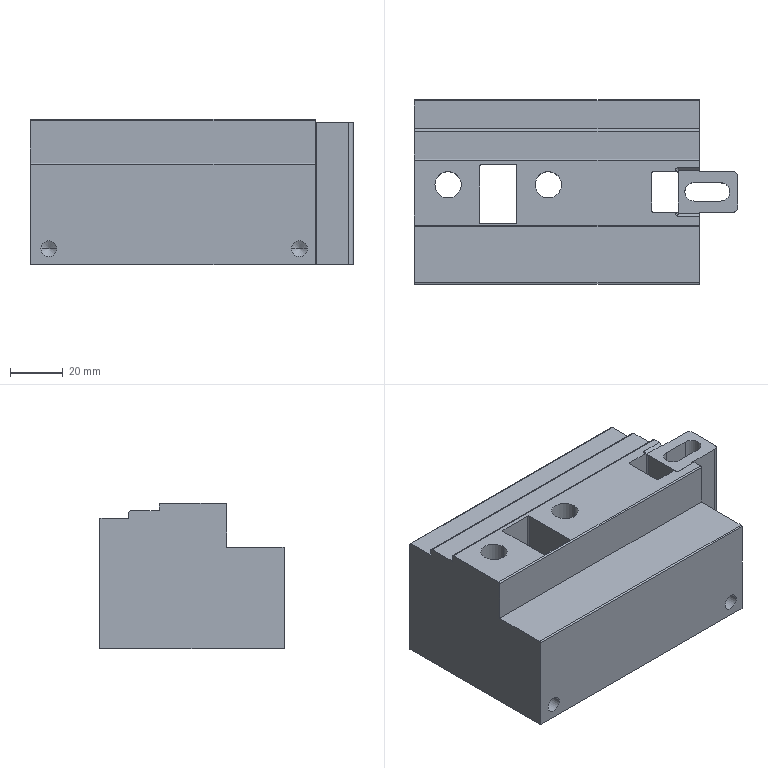Part | STEP file | KHUON DUONG_2 | 1 solid | 85 faces | box 122.5 x 70 x 55 mm | volume 306755 mm3 | cylinder 40 | plane 35 | cone 10 | commonest cylinder face diameters 1 x12 6 x8 18 x8 10 x4 7 x3 0.6 x2